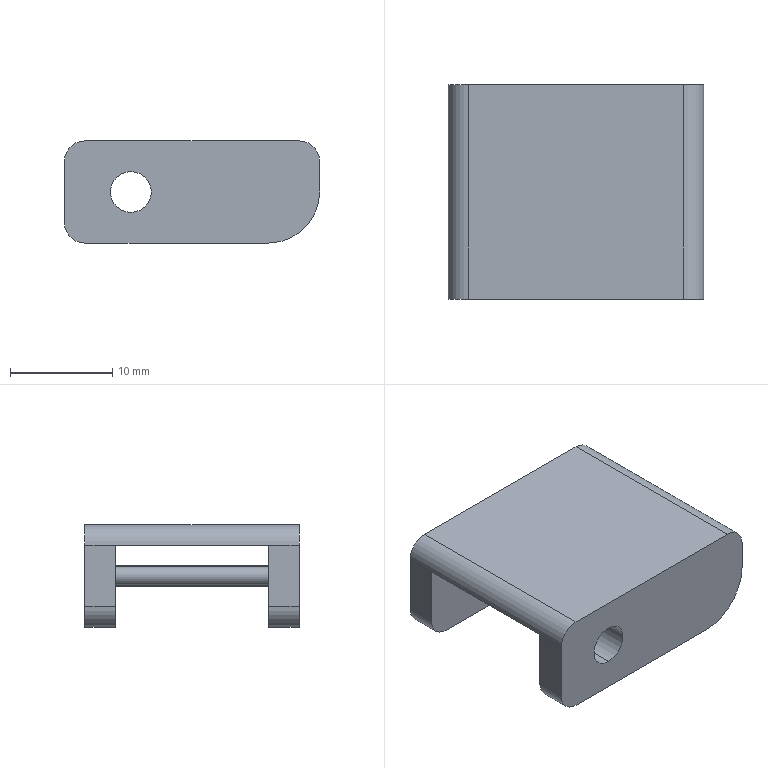Part | SolidWorks | features ICE 4, Fillet 2, Extrusion 1 | 1 solid | 26 faces | box 25 x 21 x 10 mm | volume 2190 mm3 | cylinder 14 | plane 12 | commonest cylinder face diameters 4 x8 1.809 x2 2.072 x2 10 x2
STEP:
#1=CARTESIAN_POINT('',(0.,7.5,-0.9044));
#2=VERTEX_POINT('',#1);
#3=CARTESIAN_POINT('',(0.,7.5,0.9044));
#4=VERTEX_POINT('',#3);
#5=CARTESIAN_POINT('',(0.,7.5,0.));
#6=DIRECTION('',(0.,-1.,0.));
#7=DIRECTION('',(0.,0.,1.));
#8=AXIS2_PLACEMENT_3D('',#5,#6,#7);
#9=CIRCLE('',#8,0.9044);
#10=EDGE_CURVE('',#2,#4,#9,.T.);
#11=ORIENTED_EDGE('',*,*,#10,.T.);
#12=CARTESIAN_POINT('',(0.,-7.5,0.9044));
#13=VERTEX_POINT('',#12);
#14=CARTESIAN_POINT('',(0.,10.058,0.9044));
#15=DIRECTION('',(0.,-1.,0.));
#16=VECTOR('',#15,1000.);
#17=LINE('',#14,#16);
#18=EDGE_CURVE('',#4,#13,#17,.T.);
#19=ORIENTED_EDGE('',*,*,#18,.T.);
#20=CARTESIAN_POINT('',(0.,-7.5,-0.9044));
#21=VERTEX_POINT('',#20);
#22=CARTESIAN_POINT('',(0.,-7.5,0.));
#23=DIRECTION('',(0.,1.,0.));
#24=DIRECTION('',(0.,0.,-1.));
#25=AXIS2_PLACEMENT_3D('',#22,#23,#24);
#26=CIRCLE('',#25,0.9044);
#27=EDGE_CURVE('',#13,#21,#26,.T.);
#28=ORIENTED_EDGE('',*,*,#27,.T.);
#29=CARTESIAN_POINT('',(0.,10.058,-0.9044));
#30=DIRECTION('',(0.,-1.,0.));
#31=VECTOR('',#30,1000.);
#32=LINE('',#29,#31);
#33=EDGE_CURVE('',#2,#21,#32,.T.);
#34=ORIENTED_EDGE('',*,*,#33,.F.);
#35=EDGE_LOOP('',(#11,#19,#28,#34));
#36=FACE_OUTER_BOUND('',#35,.T.);
#37=CARTESIAN_POINT('',(0.,10.058,0.));
#38=DIRECTION('',(0.,-1.,0.));
#39=DIRECTION('',(0.,0.,-1.));
#40=AXIS2_PLACEMENT_3D('',#37,#38,#39);
#41=CYLINDRICAL_SURFACE('',#40,0.9044);
#42=ADVANCED_FACE('',(#36),#41,.T.);
#43=CARTESIAN_POINT('',(4.,-7.5,1.036));
#44=VERTEX_POINT('',#43);
#45=CARTESIAN_POINT('',(4.,-7.5,-1.036));
#46=VERTEX_POINT('',#45);
#47=CARTESIAN_POINT('',(4.,-7.5,0.));
#48=DIRECTION('',(0.,1.,0.));
#49=DIRECTION('',(0.,0.,-1.));
#50=AXIS2_PLACEMENT_3D('',#47,#48,#49);
#51=CIRCLE('',#50,1.036);
#52=EDGE_CURVE('',#44,#46,#51,.T.);
#53=ORIENTED_EDGE('',*,*,#52,.T.);
#54=CARTESIAN_POINT('',(4.,7.5,-1.036));
#55=VERTEX_POINT('',#54);
#56=CARTESIAN_POINT('',(4.,-10.43,-1.036));
#57=DIRECTION('',(0.,1.,0.));
#58=VECTOR('',#57,1000.);
#59=LINE('',#56,#58);
#60=EDGE_CURVE('',#46,#55,#59,.T.);
#61=ORIENTED_EDGE('',*,*,#60,.T.);
#62=CARTESIAN_POINT('',(4.,7.5,1.036));
#63=VERTEX_POINT('',#62);
#64=CARTESIAN_POINT('',(4.,7.5,0.));
#65=DIRECTION('',(0.,1.,0.));
#66=DIRECTION('',(0.,0.,1.));
#67=AXIS2_PLACEMENT_3D('',#64,#65,#66);
#68=CIRCLE('',#67,1.036);
#69=EDGE_CURVE('',#63,#55,#68,.T.);
#70=ORIENTED_EDGE('',*,*,#69,.F.);
#71=CARTESIAN_POINT('',(4.,-10.43,1.036));
#72=DIRECTION('',(0.,1.,0.));
#73=VECTOR('',#72,1000.);
#74=LINE('',#71,#73);
#75=EDGE_CURVE('',#44,#63,#74,.T.);
#76=ORIENTED_EDGE('',*,*,#75,.F.);
#77=EDGE_LOOP('',(#53,#61,#70,#76));
#78=FACE_OUTER_BOUND('',#77,.T.);
#79=CARTESIAN_POINT('',(4.,-10.43,0.));
#80=DIRECTION('',(0.,1.,0.));
#81=DIRECTION('',(0.,0.,1.));
#82=AXIS2_PLACEMENT_3D('',#79,#80,#81);
#83=CYLINDRICAL_SURFACE('',#82,1.036);
#84=ADVANCED_FACE('',(#78),#83,.T.);
#85=CARTESIAN_POINT('',(-6.,-10.5,-2.));
#86=VERTEX_POINT('',#85);
#87=CARTESIAN_POINT('',(-6.,-10.5,2.));
#88=VERTEX_POINT('',#87);
#89=CARTESIAN_POINT('',(-6.,-10.5,0.));
#90=DIRECTION('',(0.,1.,0.));
#91=DIRECTION('',(0.,0.,1.));
#92=AXIS2_PLACEMENT_3D('',#89,#90,#91);
#93=CIRCLE('',#92,2.);
#94=EDGE_CURVE('',#86,#88,#93,.T.);
#95=ORIENTED_EDGE('',*,*,#94,.F.);
#96=CARTESIAN_POINT('',(-6.,-7.5,-2.));
#97=VERTEX_POINT('',#96);
#98=CARTESIAN_POINT('',(-6.,-10.5,-2.));
#99=DIRECTION('',(0.,1.,0.));
#100=VECTOR('',#99,1000.);
#101=LINE('',#98,#100);
#102=EDGE_CURVE('',#86,#97,#101,.T.);
#103=ORIENTED_EDGE('',*,*,#102,.T.);
#104=CARTESIAN_POINT('',(-6.,-7.5,2.));
#105=VERTEX_POINT('',#104);
#106=CARTESIAN_POINT('',(-6.,-7.5,0.));
#107=DIRECTION('',(0.,-1.,0.));
#108=DIRECTION('',(0.,0.,-1.));
#109=AXIS2_PLACEMENT_3D('',#106,#107,#108);
#110=CIRCLE('',#109,2.);
#111=EDGE_CURVE('',#105,#97,#110,.T.);
#112=ORIENTED_EDGE('',*,*,#111,.F.);
#113=CARTESIAN_POINT('',(-6.,-10.5,2.));
#114=DIRECTION('',(0.,1.,0.));
#115=VECTOR('',#114,1000.);
#116=LINE('',#113,#115);
#117=EDGE_CURVE('',#88,#105,#116,.T.);
#118=ORIENTED_EDGE('',*,*,#117,.F.);
#119=EDGE_LOOP('',(#95,#103,#112,#118));
#120=FACE_OUTER_BOUND('',#119,.T.);
#121=CARTESIAN_POINT('',(-6.,-10.5,0.));
#122=DIRECTION('',(0.,1.,0.));
#123=DIRECTION('',(0.,0.,1.));
#124=AXIS2_PLACEMENT_3D('',#121,#122,#123);
#125=CYLINDRICAL_SURFACE('',#124,2.);
#126=ADVANCED_FACE('',(#120),#125,.F.);
#127=CARTESIAN_POINT('',(-6.,7.5,-2.));
#128=VERTEX_POINT('',#127);
#129=CARTESIAN_POINT('',(-6.,7.5,2.));
#130=VERTEX_POINT('',#129);
#131=CARTESIAN_POINT('',(-6.,7.5,0.));
#132=DIRECTION('',(0.,1.,0.));
#133=DIRECTION('',(0.,0.,1.));
#134=AXIS2_PLACEMENT_3D('',#131,#132,#133);
#135=CIRCLE('',#134,2.);
#136=EDGE_CURVE('',#128,#130,#135,.T.);
#137=ORIENTED_EDGE('',*,*,#136,.F.);
#138=CARTESIAN_POINT('',(-6.,10.5,-2.));
#139=VERTEX_POINT('',#138);
#140=CARTESIAN_POINT('',(-6.,-10.5,-2.));
#141=DIRECTION('',(0.,1.,0.));
#142=VECTOR('',#141,1000.);
#143=LINE('',#140,#142);
#144=EDGE_CURVE('',#128,#139,#143,.T.);
#145=ORIENTED_EDGE('',*,*,#144,.T.);
#146=CARTESIAN_POINT('',(-6.,10.5,2.));
#147=VERTEX_POINT('',#146);
#148=CARTESIAN_POINT('',(-6.,10.5,0.));
#149=DIRECTION('',(0.,1.,0.));
#150=DIRECTION('',(0.,0.,1.));
#151=AXIS2_PLACEMENT_3D('',#148,#149,#150);
#152=CIRCLE('',#151,2.);
#153=EDGE_CURVE('',#139,#147,#152,.T.);
#154=ORIENTED_EDGE('',*,*,#153,.T.);
#155=CARTESIAN_POINT('',(-6.,-10.5,2.));
#156=DIRECTION('',(0.,1.,0.));
#157=VECTOR('',#156,1000.);
#158=LINE('',#155,#157);
#159=EDGE_CURVE('',#130,#147,#158,.T.);
#160=ORIENTED_EDGE('',*,*,#159,.F.);
#161=EDGE_LOOP('',(#137,#145,#154,#160));
#162=FACE_OUTER_BOUND('',#161,.T.);
#163=CARTESIAN_POINT('',(-6.,-10.5,0.));
#164=DIRECTION('',(0.,1.,0.));
#165=DIRECTION('',(0.,0.,1.));
#166=AXIS2_PLACEMENT_3D('',#163,#164,#165);
#167=CYLINDRICAL_SURFACE('',#166,2.);
#168=ADVANCED_FACE('',(#162),#167,.F.);
#169=CARTESIAN_POINT('',(12.5,7.5,0.));
#170=VERTEX_POINT('',#169);
#171=CARTESIAN_POINT('',(12.5,7.5,3.));
#172=VERTEX_POINT('',#171);
#173=CARTESIAN_POINT('',(12.5,7.5,-5.));
#174=DIRECTION('',(0.,0.,1.));
#175=VECTOR('',#174,1000.);
#176=LINE('',#173,#175);
#177=EDGE_CURVE('',#170,#172,#176,.T.);
#178=ORIENTED_EDGE('',*,*,#177,.F.);
#179=CARTESIAN_POINT('',(12.5,10.5,0.));
#180=VERTEX_POINT('',#179);
#181=CARTESIAN_POINT('',(12.5,10.5,0.));
#182=DIRECTION('',(0.,1.,0.));
#183=VECTOR('',#182,1000.);
#184=LINE('',#181,#183);
#185=EDGE_CURVE('',#170,#180,#184,.T.);
#186=ORIENTED_EDGE('',*,*,#185,.T.);
#187=CARTESIAN_POINT('',(12.5,10.5,3.));
#188=VERTEX_POINT('',#187);
#189=CARTESIAN_POINT('',(12.5,10.5,5.));
#190=DIRECTION('',(0.,0.,-1.));
#191=VECTOR('',#190,1000.);
#192=LINE('',#189,#191);
#193=EDGE_CURVE('',#188,#180,#192,.T.);
#194=ORIENTED_EDGE('',*,*,#193,.F.);
#195=CARTESIAN_POINT('',(12.5,10.5,3.));
#196=DIRECTION('',(0.,-1.,0.));
#197=VECTOR('',#196,1000.);
#198=LINE('',#195,#197);
#199=EDGE_CURVE('',#188,#172,#198,.T.);
#200=ORIENTED_EDGE('',*,*,#199,.T.);
#201=EDGE_LOOP('',(#178,#186,#194,#200));
#202=FACE_OUTER_BOUND('',#201,.T.);
#203=CARTESIAN_POINT('',(12.5,10.5,5.));
#204=DIRECTION('',(-1.,0.,0.));
#205=DIRECTION('',(0.,0.,1.));
#206=AXIS2_PLACEMENT_3D('',#203,#204,#205);
#207=PLANE('',#206);
#208=ADVANCED_FACE('',(#202),#207,.F.);
#209=CARTESIAN_POINT('',(-12.5,-10.5,-3.));
#210=VERTEX_POINT('',#209);
#211=CARTESIAN_POINT('',(-12.5,-10.5,3.));
#212=VERTEX_POINT('',#211);
#213=CARTESIAN_POINT('',(-12.5,-10.5,5.));
#214=DIRECTION('',(0.,0.,1.));
#215=VECTOR('',#214,1000.);
#216=LINE('',#213,#215);
#217=EDGE_CURVE('',#210,#212,#216,.T.);
#218=ORIENTED_EDGE('',*,*,#217,.T.);
#219=CARTESIAN_POINT('',(-12.5,-7.5,3.));
#220=VERTEX_POINT('',#219);
#221=CARTESIAN_POINT('',(-12.5,10.5,3.));
#222=DIRECTION('',(0.,1.,0.));
#223=VECTOR('',#222,1000.);
#224=LINE('',#221,#223);
#225=EDGE_CURVE('',#212,#220,#224,.T.);
#226=ORIENTED_EDGE('',*,*,#225,.T.);
#227=CARTESIAN_POINT('',(-12.5,-7.5,-3.));
#228=VERTEX_POINT('',#227);
#229=CARTESIAN_POINT('',(-12.5,-7.5,-5.));
#230=DIRECTION('',(0.,0.,-1.));
#231=VECTOR('',#230,1000.);
#232=LINE('',#229,#231);
#233=EDGE_CURVE('',#220,#228,#232,.T.);
#234=ORIENTED_EDGE('',*,*,#233,.T.);
#235=CARTESIAN_POINT('',(-12.5,10.5,-3.));
#236=DIRECTION('',(0.,-1.,0.));
#237=VECTOR('',#236,1000.);
#238=LINE('',#235,#237);
#239=EDGE_CURVE('',#228,#210,#238,.T.);
#240=ORIENTED_EDGE('',*,*,#239,.T.);
#241=EDGE_LOOP('',(#218,#226,#234,#240));
#242=FACE_OUTER_BOUND('',#241,.T.);
#243=CARTESIAN_POINT('',(-12.5,10.5,5.));
#244=DIRECTION('',(1.,0.,0.));
#245=DIRECTION('',(0.,0.,-1.));
#246=AXIS2_PLACEMENT_3D('',#243,#244,#245);
#247=PLANE('',#246);
#248=ADVANCED_FACE('',(#242),#247,.F.);
#249=CARTESIAN_POINT('',(-10.5,-7.5,-5.));
#250=VERTEX_POINT('',#249);
#251=CARTESIAN_POINT('',(7.5,-7.5,-5.));
#252=VERTEX_POINT('',#251);
#253=CARTESIAN_POINT('',(-12.5,-7.5,-5.));
#254=DIRECTION('',(1.,0.,0.));
#255=VECTOR('',#254,1000.);
#256=LINE('',#253,#255);
#257=EDGE_CURVE('',#250,#252,#256,.T.);
#258=ORIENTED_EDGE('',*,*,#257,.T.);
#259=CARTESIAN_POINT('',(7.5,-10.5,-5.));
#260=VERTEX_POINT('',#259);
#261=CARTESIAN_POINT('',(7.5,10.5,-5.));
#262=DIRECTION('',(0.,-1.,0.));
#263=VECTOR('',#262,1000.);
#264=LINE('',#261,#263);
#265=EDGE_CURVE('',#252,#260,#264,.T.);
#266=ORIENTED_EDGE('',*,*,#265,.T.);
#267=CARTESIAN_POINT('',(-10.5,-10.5,-5.));
#268=VERTEX_POINT('',#267);
#269=CARTESIAN_POINT('',(-12.5,-10.5,-5.));
#270=DIRECTION('',(-1.,0.,0.));
#271=VECTOR('',#270,1000.);
#272=LINE('',#269,#271);
#273=EDGE_CURVE('',#260,#268,#272,.T.);
#274=ORIENTED_EDGE('',*,*,#273,.T.);
#275=CARTESIAN_POINT('',(-10.5,10.5,-5.));
#276=DIRECTION('',(0.,1.,0.));
#277=VECTOR('',#276,1000.);
#278=LINE('',#275,#277);
#279=EDGE_CURVE('',#268,#250,#278,.T.);
#280=ORIENTED_EDGE('',*,*,#279,.T.);
#281=EDGE_LOOP('',(#258,#266,#274,#280));
#282=FACE_OUTER_BOUND('',#281,.T.);
#283=CARTESIAN_POINT('',(-12.5,10.5,-5.));
#284=DIRECTION('',(0.,0.,1.));
#285=DIRECTION('',(1.,0.,0.));
#286=AXIS2_PLACEMENT_3D('',#283,#284,#285);
#287=PLANE('',#286);
#288=ADVANCED_FACE('',(#282),#287,.F.);
#289=CARTESIAN_POINT('',(12.5,-10.5,3.));
#290=VERTEX_POINT('',#289);
#291=CARTESIAN_POINT('',(12.5,-10.5,0.));
#292=VERTEX_POINT('',#291);
#293=CARTESIAN_POINT('',(12.5,-10.5,5.));
#294=DIRECTION('',(0.,0.,-1.));
#295=VECTOR('',#294,1000.);
#296=LINE('',#293,#295);
#297=EDGE_CURVE('',#290,#292,#296,.T.);
#298=ORIENTED_EDGE('',*,*,#297,.T.);
#299=CARTESIAN_POINT('',(12.5,-7.5,0.));
#300=VERTEX_POINT('',#299);
#301=CARTESIAN_POINT('',(12.5,10.5,0.));
#302=DIRECTION('',(0.,1.,0.));
#303=VECTOR('',#302,1000.);
#304=LINE('',#301,#303);
#305=EDGE_CURVE('',#292,#300,#304,.T.);
#306=ORIENTED_EDGE('',*,*,#305,.T.);
#307=CARTESIAN_POINT('',(12.5,-7.5,3.));
#308=VERTEX_POINT('',#307);
#309=CARTESIAN_POINT('',(12.5,-7.5,-5.));
#310=DIRECTION('',(0.,0.,-1.));
#311=VECTOR('',#310,1000.);
#312=LINE('',#309,#311);
#313=EDGE_CURVE('',#308,#300,#312,.T.);
#314=ORIENTED_EDGE('',*,*,#313,.F.);
#315=CARTESIAN_POINT('',(12.5,10.5,3.));
#316=DIRECTION('',(0.,-1.,0.));
#317=VECTOR('',#316,1000.);
#318=LINE('',#315,#317);
#319=EDGE_CURVE('',#308,#290,#318,.T.);
#320=ORIENTED_EDGE('',*,*,#319,.T.);
#321=EDGE_LOOP('',(#298,#306,#314,#320));
#322=FACE_OUTER_BOUND('',#321,.T.);
#323=CARTESIAN_POINT('',(12.5,10.5,5.));
#324=DIRECTION('',(-1.,0.,0.));
#325=DIRECTION('',(0.,0.,1.));
#326=AXIS2_PLACEMENT_3D('',#323,#324,#325);
#327=PLANE('',#326);
#328=ADVANCED_FACE('',(#322),#327,.F.);
#329=CARTESIAN_POINT('',(7.5,10.5,-5.));
#330=VERTEX_POINT('',#329);
#331=CARTESIAN_POINT('',(-10.5,10.5,-5.));
#332=VERTEX_POINT('',#331);
#333=CARTESIAN_POINT('',(-12.5,10.5,-5.));
#334=DIRECTION('',(-1.,0.,0.));
#335=VECTOR('',#334,1000.);
#336=LINE('',#333,#335);
#337=EDGE_CURVE('',#330,#332,#336,.T.);
#338=ORIENTED_EDGE('',*,*,#337,.F.);
#339=CARTESIAN_POINT('',(7.5,7.5,-5.));
#340=VERTEX_POINT('',#339);
#341=CARTESIAN_POINT('',(7.5,10.5,-5.));
#342=DIRECTION('',(0.,-1.,0.));
#343=VECTOR('',#342,1000.);
#344=LINE('',#341,#343);
#345=EDGE_CURVE('',#330,#340,#344,.T.);
#346=ORIENTED_EDGE('',*,*,#345,.T.);
#347=CARTESIAN_POINT('',(-10.5,7.5,-5.));
#348=VERTEX_POINT('',#347);
#349=CARTESIAN_POINT('',(-12.5,7.5,-5.));
#350=DIRECTION('',(1.,0.,0.));
#351=VECTOR('',#350,1000.);
#352=LINE('',#349,#351);
#353=EDGE_CURVE('',#348,#340,#352,.T.);
#354=ORIENTED_EDGE('',*,*,#353,.F.);
#355=CARTESIAN_POINT('',(-10.5,10.5,-5.));
#356=DIRECTION('',(0.,1.,0.));
#357=VECTOR('',#356,1000.);
#358=LINE('',#355,#357);
#359=EDGE_CURVE('',#348,#332,#358,.T.);
#360=ORIENTED_EDGE('',*,*,#359,.T.);
#361=EDGE_LOOP('',(#338,#346,#354,#360));
#362=FACE_OUTER_BOUND('',#361,.T.);
#363=CARTESIAN_POINT('',(-12.5,10.5,-5.));
#364=DIRECTION('',(0.,0.,1.));
#365=DIRECTION('',(1.,0.,0.));
#366=AXIS2_PLACEMENT_3D('',#363,#364,#365);
#367=PLANE('',#366);
#368=ADVANCED_FACE('',(#362),#367,.F.);
#369=CARTESIAN_POINT('',(-12.5,7.5,-3.));
#370=VERTEX_POINT('',#369);
#371=CARTESIAN_POINT('',(-12.5,7.5,3.));
#372=VERTEX_POINT('',#371);
#373=CARTESIAN_POINT('',(-12.5,7.5,-5.));
#374=DIRECTION('',(0.,0.,1.));
#375=VECTOR('',#374,1000.);
#376=LINE('',#373,#375);
#377=EDGE_CURVE('',#370,#372,#376,.T.);
#378=ORIENTED_EDGE('',*,*,#377,.T.);
#379=CARTESIAN_POINT('',(-12.5,10.5,3.));
#380=VERTEX_POINT('',#379);
#381=CARTESIAN_POINT('',(-12.5,10.5,3.));
#382=DIRECTION('',(0.,1.,0.));
#383=VECTOR('',#382,1000.);
#384=LINE('',#381,#383);
#385=EDGE_CURVE('',#372,#380,#384,.T.);
#386=ORIENTED_EDGE('',*,*,#385,.T.);
#387=CARTESIAN_POINT('',(-12.5,10.5,-3.));
#388=VERTEX_POINT('',#387);
#389=CARTESIAN_POINT('',(-12.5,10.5,5.));
#390=DIRECTION('',(0.,0.,1.));
#391=VECTOR('',#390,1000.);
#392=LINE('',#389,#391);
#393=EDGE_CURVE('',#388,#380,#392,.T.);
#394=ORIENTED_EDGE('',*,*,#393,.F.);
#395=CARTESIAN_POINT('',(-12.5,10.5,-3.));
#396=DIRECTION('',(0.,-1.,0.));
#397=VECTOR('',#396,1000.);
#398=LINE('',#395,#397);
#399=EDGE_CURVE('',#388,#370,#398,.T.);
#400=ORIENTED_EDGE('',*,*,#399,.T.);
#401=EDGE_LOOP('',(#378,#386,#394,#400));
#402=FACE_OUTER_BOUND('',#401,.T.);
#403=CARTESIAN_POINT('',(-12.5,10.5,5.));
#404=DIRECTION('',(1.,0.,0.));
#405=DIRECTION('',(0.,0.,-1.));
#406=AXIS2_PLACEMENT_3D('',#403,#404,#405);
#407=PLANE('',#406);
#408=ADVANCED_FACE('',(#402),#407,.F.);
#409=CARTESIAN_POINT('',(-10.5,10.5,5.));
#410=VERTEX_POINT('',#409);
#411=CARTESIAN_POINT('',(10.5,10.5,5.));
#412=VERTEX_POINT('',#411);
#413=CARTESIAN_POINT('',(-12.5,10.5,5.));
#414=DIRECTION('',(1.,0.,0.));
#415=VECTOR('',#414,1000.);
#416=LINE('',#413,#415);
#417=EDGE_CURVE('',#410,#412,#416,.T.);
#418=ORIENTED_EDGE('',*,*,#417,.F.);
#419=CARTESIAN_POINT('',(-10.5,-10.5,5.));
#420=VERTEX_POINT('',#419);
#421=CARTESIAN_POINT('',(-10.5,10.5,5.));
#422=DIRECTION('',(0.,-1.,0.));
#423=VECTOR('',#422,1000.);
#424=LINE('',#421,#423);
#425=EDGE_CURVE('',#410,#420,#424,.T.);
#426=ORIENTED_EDGE('',*,*,#425,.T.);
#427=CARTESIAN_POINT('',(10.5,-10.5,5.));
#428=VERTEX_POINT('',#427);
#429=CARTESIAN_POINT('',(-12.5,-10.5,5.));
#430=DIRECTION('',(1.,0.,0.));
#431=VECTOR('',#430,1000.);
#432=LINE('',#429,#431);
#433=EDGE_CURVE('',#420,#428,#432,.T.);
#434=ORIENTED_EDGE('',*,*,#433,.T.);
#435=CARTESIAN_POINT('',(10.5,10.5,5.));
#436=DIRECTION('',(0.,1.,0.));
#437=VECTOR('',#436,1000.);
#438=LINE('',#435,#437);
#439=EDGE_CURVE('',#428,#412,#438,.T.);
#440=ORIENTED_EDGE('',*,*,#439,.T.);
#441=EDGE_LOOP('',(#418,#426,#434,#440));
#442=FACE_OUTER_BOUND('',#441,.T.);
#443=CARTESIAN_POINT('',(-12.5,10.5,5.));
#444=DIRECTION('',(0.,0.,-1.));
#445=DIRECTION('',(-1.,0.,0.));
#446=AXIS2_PLACEMENT_3D('',#443,#444,#445);
#447=PLANE('',#446);
#448=ADVANCED_FACE('',(#442),#447,.F.);
#449=CARTESIAN_POINT('',(-6.,10.5,0.));
#450=DIRECTION('',(0.,1.,0.));
#451=DIRECTION('',(0.,0.,1.));
#452=AXIS2_PLACEMENT_3D('',#449,#450,#451);
#453=CIRCLE('',#452,2.);
#454=EDGE_CURVE('',#147,#139,#453,.T.);
#455=ORIENTED_EDGE('',*,*,#454,.F.);
#456=ORIENTED_EDGE('',*,*,#153,.F.);
#457=EDGE_LOOP('',(#455,#456));
#458=FACE_BOUND('',#457,.T.);
#459=ORIENTED_EDGE('',*,*,#193,.T.);
#460=CARTESIAN_POINT('',(7.5,10.5,0.));
#461=DIRECTION('',(0.,1.,0.));
#462=DIRECTION('',(0.,0.,-1.));
#463=AXIS2_PLACEMENT_3D('',#460,#461,#462);
#464=CIRCLE('',#463,5.);
#465=EDGE_CURVE('',#180,#330,#464,.T.);
#466=ORIENTED_EDGE('',*,*,#465,.T.);
#467=ORIENTED_EDGE('',*,*,#337,.T.);
#468=CARTESIAN_POINT('',(-10.5,10.5,-3.));
#469=DIRECTION('',(0.,1.,0.));
#470=DIRECTION('',(0.,0.,-1.));
#471=AXIS2_PLACEMENT_3D('',#468,#469,#470);
#472=CIRCLE('',#471,2.);
#473=EDGE_CURVE('',#332,#388,#472,.T.);
#474=ORIENTED_EDGE('',*,*,#473,.T.);
#475=ORIENTED_EDGE('',*,*,#393,.T.);
#476=CARTESIAN_POINT('',(-10.5,10.5,3.));
#477=DIRECTION('',(0.,1.,0.));
#478=DIRECTION('',(0.,0.,-1.));
#479=AXIS2_PLACEMENT_3D('',#476,#477,#478);
#480=CIRCLE('',#479,2.);
#481=EDGE_CURVE('',#380,#410,#480,.T.);
#482=ORIENTED_EDGE('',*,*,#481,.T.);
#483=ORIENTED_EDGE('',*,*,#417,.T.);
#484=CARTESIAN_POINT('',(10.5,10.5,3.));
#485=DIRECTION('',(0.,1.,0.));
#486=DIRECTION('',(0.,0.,-1.));
#487=AXIS2_PLACEMENT_3D('',#484,#485,#486);
#488=CIRCLE('',#487,2.);
#489=EDGE_CURVE('',#412,#188,#488,.T.);
#490=ORIENTED_EDGE('',*,*,#489,.T.);
#491=EDGE_LOOP('',(#459,#466,#467,#474,#475,#482,#483,#490));
#492=FACE_OUTER_BOUND('',#491,.T.);
#493=CARTESIAN_POINT('',(0.,10.5,0.));
#494=DIRECTION('',(0.,-1.,0.));
#495=DIRECTION('',(0.,0.,-1.));
#496=AXIS2_PLACEMENT_3D('',#493,#494,#495);
#497=PLANE('',#496);
#498=ADVANCED_FACE('',(#458,#492),#497,.F.);
#499=CARTESIAN_POINT('',(-6.,-10.5,0.));
#500=DIRECTION('',(0.,1.,0.));
#501=DIRECTION('',(0.,0.,1.));
#502=AXIS2_PLACEMENT_3D('',#499,#500,#501);
#503=CIRCLE('',#502,2.);
#504=EDGE_CURVE('',#88,#86,#503,.T.);
#505=ORIENTED_EDGE('',*,*,#504,.T.);
#506=ORIENTED_EDGE('',*,*,#94,.T.);
#507=EDGE_LOOP('',(#505,#506));
#508=FACE_BOUND('',#507,.T.);
#509=ORIENTED_EDGE('',*,*,#273,.F.);
#510=CARTESIAN_POINT('',(7.5,-10.5,0.));
#511=DIRECTION('',(0.,-1.,0.));
#512=DIRECTION('',(0.,0.,-1.));
#513=AXIS2_PLACEMENT_3D('',#510,#511,#512);
#514=CIRCLE('',#513,5.);
#515=EDGE_CURVE('',#260,#292,#514,.T.);
#516=ORIENTED_EDGE('',*,*,#515,.T.);
#517=ORIENTED_EDGE('',*,*,#297,.F.);
#518=CARTESIAN_POINT('',(10.5,-10.5,3.));
#519=DIRECTION('',(0.,-1.,0.));
#520=DIRECTION('',(0.,0.,-1.));
#521=AXIS2_PLACEMENT_3D('',#518,#519,#520);
#522=CIRCLE('',#521,2.);
#523=EDGE_CURVE('',#290,#428,#522,.T.);
#524=ORIENTED_EDGE('',*,*,#523,.T.);
#525=ORIENTED_EDGE('',*,*,#433,.F.);
#526=CARTESIAN_POINT('',(-10.5,-10.5,3.));
#527=DIRECTION('',(0.,-1.,0.));
#528=DIRECTION('',(0.,0.,-1.));
#529=AXIS2_PLACEMENT_3D('',#526,#527,#528);
#530=CIRCLE('',#529,2.);
#531=EDGE_CURVE('',#420,#212,#530,.T.);
#532=ORIENTED_EDGE('',*,*,#531,.T.);
#533=ORIENTED_EDGE('',*,*,#217,.F.);
#534=CARTESIAN_POINT('',(-10.5,-10.5,-3.));
#535=DIRECTION('',(0.,-1.,0.));
#536=DIRECTION('',(0.,0.,-1.));
#537=AXIS2_PLACEMENT_3D('',#534,#535,#536);
#538=CIRCLE('',#537,2.);
#539=EDGE_CURVE('',#210,#268,#538,.T.);
#540=ORIENTED_EDGE('',*,*,#539,.T.);
#541=EDGE_LOOP('',(#509,#516,#517,#524,#525,#532,#533,#540));
#542=FACE_OUTER_BOUND('',#541,.T.);
#543=CARTESIAN_POINT('',(0.,-10.5,0.));
#544=DIRECTION('',(0.,-1.,0.));
#545=DIRECTION('',(0.,0.,-1.));
#546=AXIS2_PLACEMENT_3D('',#543,#544,#545);
#547=PLANE('',#546);
#548=ADVANCED_FACE('',(#508,#542),#547,.T.);
#549=CARTESIAN_POINT('',(0.,-7.5,0.));
#550=DIRECTION('',(0.,1.,0.));
#551=DIRECTION('',(0.,0.,-1.));
#552=AXIS2_PLACEMENT_3D('',#549,#550,#551);
#553=CIRCLE('',#552,0.9044);
#554=EDGE_CURVE('',#21,#13,#553,.T.);
#555=ORIENTED_EDGE('',*,*,#554,.F.);
#556=ORIENTED_EDGE('',*,*,#27,.F.);
#557=EDGE_LOOP('',(#555,#556));
#558=FACE_BOUND('',#557,.T.);
#559=ORIENTED_EDGE('',*,*,#52,.F.);
#560=CARTESIAN_POINT('',(4.,-7.5,0.));
#561=DIRECTION('',(0.,1.,0.));
#562=DIRECTION('',(0.,0.,-1.));
#563=AXIS2_PLACEMENT_3D('',#560,#561,#562);
#564=CIRCLE('',#563,1.036);
#565=EDGE_CURVE('',#46,#44,#564,.T.);
#566=ORIENTED_EDGE('',*,*,#565,.F.);
#567=EDGE_LOOP('',(#559,#566));
#568=FACE_BOUND('',#567,.T.);
#569=ORIENTED_EDGE('',*,*,#111,.T.);
#570=CARTESIAN_POINT('',(-6.,-7.5,0.));
#571=DIRECTION('',(0.,-1.,0.));
#572=DIRECTION('',(0.,0.,-1.));
#573=AXIS2_PLACEMENT_3D('',#570,#571,#572);
#574=CIRCLE('',#573,2.);
#575=EDGE_CURVE('',#97,#105,#574,.T.);
#576=ORIENTED_EDGE('',*,*,#575,.T.);
#577=EDGE_LOOP('',(#569,#576));
#578=FACE_BOUND('',#577,.T.);
#579=ORIENTED_EDGE('',*,*,#313,.T.);
#580=CARTESIAN_POINT('',(7.5,-7.5,0.));
#581=DIRECTION('',(0.,1.,0.));
#582=DIRECTION('',(0.,0.,-1.));
#583=AXIS2_PLACEMENT_3D('',#580,#581,#582);
#584=CIRCLE('',#583,5.);
#585=EDGE_CURVE('',#300,#252,#584,.T.);
#586=ORIENTED_EDGE('',*,*,#585,.T.);
#587=ORIENTED_EDGE('',*,*,#257,.F.);
#588=CARTESIAN_POINT('',(-10.5,-7.5,-3.));
#589=DIRECTION('',(0.,1.,0.));
#590=DIRECTION('',(0.,0.,-1.));
#591=AXIS2_PLACEMENT_3D('',#588,#589,#590);
#592=CIRCLE('',#591,2.);
#593=EDGE_CURVE('',#250,#228,#592,.T.);
#594=ORIENTED_EDGE('',*,*,#593,.T.);
#595=ORIENTED_EDGE('',*,*,#233,.F.);
#596=CARTESIAN_POINT('',(-12.5,-7.5,3.));
#597=DIRECTION('',(1.,0.,0.));
#598=VECTOR('',#597,1000.);
#599=LINE('',#596,#598);
#600=EDGE_CURVE('',#220,#308,#599,.T.);
#601=ORIENTED_EDGE('',*,*,#600,.T.);
#602=EDGE_LOOP('',(#579,#586,#587,#594,#595,#601));
#603=FACE_OUTER_BOUND('',#602,.T.);
#604=CARTESIAN_POINT('',(-12.5,-7.5,-5.));
#605=DIRECTION('',(0.,-1.,0.));
#606=DIRECTION('',(0.,0.,-1.));
#607=AXIS2_PLACEMENT_3D('',#604,#605,#606);
#608=PLANE('',#607);
#609=ADVANCED_FACE('',(#558,#568,#578,#603),#608,.F.);
#610=CARTESIAN_POINT('',(12.5,-7.5,3.));
#611=DIRECTION('',(0.,-1.,0.));
#612=VECTOR('',#611,1000.);
#613=LINE('',#610,#612);
#614=EDGE_CURVE('',#172,#308,#613,.T.);
#615=ORIENTED_EDGE('',*,*,#614,.T.);
#616=ORIENTED_EDGE('',*,*,#600,.F.);
#617=CARTESIAN_POINT('',(-12.5,-7.5,3.));
#618=DIRECTION('',(0.,-1.,0.));
#619=VECTOR('',#618,1000.);
#620=LINE('',#617,#619);
#621=EDGE_CURVE('',#372,#220,#620,.T.);
#622=ORIENTED_EDGE('',*,*,#621,.F.);
#623=CARTESIAN_POINT('',(-12.5,7.5,3.));
#624=DIRECTION('',(1.,0.,0.));
#625=VECTOR('',#624,1000.);
#626=LINE('',#623,#625);
#627=EDGE_CURVE('',#372,#172,#626,.T.);
#628=ORIENTED_EDGE('',*,*,#627,.T.);
#629=EDGE_LOOP('',(#615,#616,#622,#628));
#630=FACE_OUTER_BOUND('',#629,.T.);
#631=CARTESIAN_POINT('',(-12.5,-7.5,3.));
#632=DIRECTION('',(0.,0.,1.));
#633=DIRECTION('',(1.,0.,0.));
#634=AXIS2_PLACEMENT_3D('',#631,#632,#633);
#635=PLANE('',#634);
#636=ADVANCED_FACE('',(#630),#635,.F.);
#637=ORIENTED_EDGE('',*,*,#10,.F.);
#638=CARTESIAN_POINT('',(0.,7.5,0.));
#639=DIRECTION('',(0.,-1.,0.));
#640=DIRECTION('',(0.,0.,1.));
#641=AXIS2_PLACEMENT_3D('',#638,#639,#640);
#642=CIRCLE('',#641,0.9044);
#643=EDGE_CURVE('',#4,#2,#642,.T.);
#644=ORIENTED_EDGE('',*,*,#643,.F.);
#645=EDGE_LOOP('',(#637,#644));
#646=FACE_BOUND('',#645,.T.);
#647=ORIENTED_EDGE('',*,*,#69,.T.);
#648=CARTESIAN_POINT('',(4.,7.5,0.));
#649=DIRECTION('',(0.,1.,0.));
#650=DIRECTION('',(0.,0.,1.));
#651=AXIS2_PLACEMENT_3D('',#648,#649,#650);
#652=CIRCLE('',#651,1.036);
#653=EDGE_CURVE('',#55,#63,#652,.T.);
#654=ORIENTED_EDGE('',*,*,#653,.T.);
#655=EDGE_LOOP('',(#647,#654));
#656=FACE_BOUND('',#655,.T.);
#657=CARTESIAN_POINT('',(-6.,7.5,0.));
#658=DIRECTION('',(0.,1.,0.));
#659=DIRECTION('',(0.,0.,1.));
#660=AXIS2_PLACEMENT_3D('',#657,#658,#659);
#661=CIRCLE('',#660,2.);
#662=EDGE_CURVE('',#130,#128,#661,.T.);
#663=ORIENTED_EDGE('',*,*,#662,.T.);
#664=ORIENTED_EDGE('',*,*,#136,.T.);
#665=EDGE_LOOP('',(#663,#664));
#666=FACE_BOUND('',#665,.T.);
#667=ORIENTED_EDGE('',*,*,#353,.T.);
#668=CARTESIAN_POINT('',(7.5,7.5,0.));
#669=DIRECTION('',(0.,-1.,0.));
#670=DIRECTION('',(0.,0.,1.));
#671=AXIS2_PLACEMENT_3D('',#668,#669,#670);
#672=CIRCLE('',#671,5.);
#673=EDGE_CURVE('',#340,#170,#672,.T.);
#674=ORIENTED_EDGE('',*,*,#673,.T.);
#675=ORIENTED_EDGE('',*,*,#177,.T.);
#676=ORIENTED_EDGE('',*,*,#627,.F.);
#677=ORIENTED_EDGE('',*,*,#377,.F.);
#678=CARTESIAN_POINT('',(-10.5,7.5,-3.));
#679=DIRECTION('',(0.,-1.,0.));
#680=DIRECTION('',(0.,0.,1.));
#681=AXIS2_PLACEMENT_3D('',#678,#679,#680);
#682=CIRCLE('',#681,2.);
#683=EDGE_CURVE('',#370,#348,#682,.T.);
#684=ORIENTED_EDGE('',*,*,#683,.T.);
#685=EDGE_LOOP('',(#667,#674,#675,#676,#677,#684));
#686=FACE_OUTER_BOUND('',#685,.T.);
#687=CARTESIAN_POINT('',(-12.5,7.5,-5.));
#688=DIRECTION('',(0.,1.,0.));
#689=DIRECTION('',(0.,0.,1.));
#690=AXIS2_PLACEMENT_3D('',#687,#688,#689);
#691=PLANE('',#690);
#692=ADVANCED_FACE('',(#646,#656,#666,#686),#691,.F.);
#693=ORIENTED_EDGE('',*,*,#621,.T.);
#694=ORIENTED_EDGE('',*,*,#225,.F.);
#695=ORIENTED_EDGE('',*,*,#531,.F.);
#696=ORIENTED_EDGE('',*,*,#425,.F.);
#697=ORIENTED_EDGE('',*,*,#481,.F.);
#698=ORIENTED_EDGE('',*,*,#385,.F.);
#699=EDGE_LOOP('',(#693,#694,#695,#696,#697,#698));
#700=FACE_OUTER_BOUND('',#699,.T.);
#701=CARTESIAN_POINT('',(-10.5,10.5,3.));
#702=DIRECTION('',(0.,-1.,0.));
#703=DIRECTION('',(0.,0.,-1.));
#704=AXIS2_PLACEMENT_3D('',#701,#702,#703);
#705=CYLINDRICAL_SURFACE('',#704,2.);
#706=ADVANCED_FACE('',(#700),#705,.T.);
#707=ORIENTED_EDGE('',*,*,#489,.F.);
#708=ORIENTED_EDGE('',*,*,#439,.F.);
#709=ORIENTED_EDGE('',*,*,#523,.F.);
#710=ORIENTED_EDGE('',*,*,#319,.F.);
#711=ORIENTED_EDGE('',*,*,#614,.F.);
#712=ORIENTED_EDGE('',*,*,#199,.F.);
#713=EDGE_LOOP('',(#707,#708,#709,#710,#711,#712));
#714=FACE_OUTER_BOUND('',#713,.T.);
#715=CARTESIAN_POINT('',(10.5,10.5,3.));
#716=DIRECTION('',(0.,-1.,0.));
#717=DIRECTION('',(0.,0.,-1.));
#718=AXIS2_PLACEMENT_3D('',#715,#716,#717);
#719=CYLINDRICAL_SURFACE('',#718,2.);
#720=ADVANCED_FACE('',(#714),#719,.T.);
#721=ORIENTED_EDGE('',*,*,#593,.F.);
#722=ORIENTED_EDGE('',*,*,#279,.F.);
#723=ORIENTED_EDGE('',*,*,#539,.F.);
#724=ORIENTED_EDGE('',*,*,#239,.F.);
#725=EDGE_LOOP('',(#721,#722,#723,#724));
#726=FACE_OUTER_BOUND('',#725,.T.);
#727=CARTESIAN_POINT('',(-10.5,10.5,-3.));
#728=DIRECTION('',(0.,-1.,0.));
#729=DIRECTION('',(0.,0.,-1.));
#730=AXIS2_PLACEMENT_3D('',#727,#728,#729);
#731=CYLINDRICAL_SURFACE('',#730,2.);
#732=ADVANCED_FACE('',(#726),#731,.T.);
#733=ORIENTED_EDGE('',*,*,#473,.F.);
#734=ORIENTED_EDGE('',*,*,#359,.F.);
#735=ORIENTED_EDGE('',*,*,#683,.F.);
#736=ORIENTED_EDGE('',*,*,#399,.F.);
#737=EDGE_LOOP('',(#733,#734,#735,#736));
#738=FACE_OUTER_BOUND('',#737,.T.);
#739=CARTESIAN_POINT('',(-10.5,10.5,-3.));
#740=DIRECTION('',(0.,-1.,0.));
#741=DIRECTION('',(0.,0.,-1.));
#742=AXIS2_PLACEMENT_3D('',#739,#740,#741);
#743=CYLINDRICAL_SURFACE('',#742,2.);
#744=ADVANCED_FACE('',(#738),#743,.T.);
#745=ORIENTED_EDGE('',*,*,#585,.F.);
#746=ORIENTED_EDGE('',*,*,#305,.F.);
#747=ORIENTED_EDGE('',*,*,#515,.F.);
#748=ORIENTED_EDGE('',*,*,#265,.F.);
#749=EDGE_LOOP('',(#745,#746,#747,#748));
#750=FACE_OUTER_BOUND('',#749,.T.);
#751=CARTESIAN_POINT('',(7.5,10.5,0.));
#752=DIRECTION('',(0.,-1.,0.));
#753=DIRECTION('',(0.,0.,-1.));
#754=AXIS2_PLACEMENT_3D('',#751,#752,#753);
#755=CYLINDRICAL_SURFACE('',#754,5.);
#756=ADVANCED_FACE('',(#750),#755,.T.);
#757=ORIENTED_EDGE('',*,*,#465,.F.);
#758=ORIENTED_EDGE('',*,*,#185,.F.);
#759=ORIENTED_EDGE('',*,*,#673,.F.);
#760=ORIENTED_EDGE('',*,*,#345,.F.);
#761=EDGE_LOOP('',(#757,#758,#759,#760));
#762=FACE_OUTER_BOUND('',#761,.T.);
#763=CARTESIAN_POINT('',(7.5,10.5,0.));
#764=DIRECTION('',(0.,-1.,0.));
#765=DIRECTION('',(0.,0.,-1.));
#766=AXIS2_PLACEMENT_3D('',#763,#764,#765);
#767=CYLINDRICAL_SURFACE('',#766,5.);
#768=ADVANCED_FACE('',(#762),#767,.T.);
#769=ORIENTED_EDGE('',*,*,#144,.F.);
#770=ORIENTED_EDGE('',*,*,#662,.F.);
#771=ORIENTED_EDGE('',*,*,#159,.T.);
#772=ORIENTED_EDGE('',*,*,#454,.T.);
#773=EDGE_LOOP('',(#769,#770,#771,#772));
#774=FACE_OUTER_BOUND('',#773,.T.);
#775=CARTESIAN_POINT('',(-6.,-10.5,0.));
#776=DIRECTION('',(0.,1.,0.));
#777=DIRECTION('',(0.,0.,1.));
#778=AXIS2_PLACEMENT_3D('',#775,#776,#777);
#779=CYLINDRICAL_SURFACE('',#778,2.);
#780=ADVANCED_FACE('',(#774),#779,.F.);
#781=ORIENTED_EDGE('',*,*,#102,.F.);
#782=ORIENTED_EDGE('',*,*,#504,.F.);
#783=ORIENTED_EDGE('',*,*,#117,.T.);
#784=ORIENTED_EDGE('',*,*,#575,.F.);
#785=EDGE_LOOP('',(#781,#782,#783,#784));
#786=FACE_OUTER_BOUND('',#785,.T.);
#787=CARTESIAN_POINT('',(-6.,-10.5,0.));
#788=DIRECTION('',(0.,1.,0.));
#789=DIRECTION('',(0.,0.,1.));
#790=AXIS2_PLACEMENT_3D('',#787,#788,#789);
#791=CYLINDRICAL_SURFACE('',#790,2.);
#792=ADVANCED_FACE('',(#786),#791,.F.);
#793=ORIENTED_EDGE('',*,*,#60,.F.);
#794=ORIENTED_EDGE('',*,*,#565,.T.);
#795=ORIENTED_EDGE('',*,*,#75,.T.);
#796=ORIENTED_EDGE('',*,*,#653,.F.);
#797=EDGE_LOOP('',(#793,#794,#795,#796));
#798=FACE_OUTER_BOUND('',#797,.T.);
#799=CARTESIAN_POINT('',(4.,-10.43,0.));
#800=DIRECTION('',(0.,1.,0.));
#801=DIRECTION('',(0.,0.,1.));
#802=AXIS2_PLACEMENT_3D('',#799,#800,#801);
#803=CYLINDRICAL_SURFACE('',#802,1.036);
#804=ADVANCED_FACE('',(#798),#803,.T.);
#805=ORIENTED_EDGE('',*,*,#18,.F.);
#806=ORIENTED_EDGE('',*,*,#643,.T.);
#807=ORIENTED_EDGE('',*,*,#33,.T.);
#808=ORIENTED_EDGE('',*,*,#554,.T.);
#809=EDGE_LOOP('',(#805,#806,#807,#808));
#810=FACE_OUTER_BOUND('',#809,.T.);
#811=CARTESIAN_POINT('',(0.,10.058,0.));
#812=DIRECTION('',(0.,-1.,0.));
#813=DIRECTION('',(0.,0.,-1.));
#814=AXIS2_PLACEMENT_3D('',#811,#812,#813);
#815=CYLINDRICAL_SURFACE('',#814,0.9044);
#816=ADVANCED_FACE('',(#810),#815,.T.);
#817=CLOSED_SHELL('',(#42,#84,#126,#168,#208,#248,#288,#328,#368,#408,#448,#498,#548,#609,#636,#692,#706,#720,#732,#744,#756,#768,#780,#792,#804,#816));
#818=MANIFOLD_SOLID_BREP('',#817);
#819=CARTESIAN_POINT('',(0.,0.,0.));
#820=DIRECTION('',(0.,0.,1.));
#821=DIRECTION('',(1.,0.,0.));
#822=AXIS2_PLACEMENT_3D('',#819,#820,#821);
#823=(LENGTH_UNIT()NAMED_UNIT(*)SI_UNIT(.MILLI.,.METRE.));
#824=UNCERTAINTY_MEASURE_WITH_UNIT(LENGTH_MEASURE(0.00001),#823,'','');
#825=(NAMED_UNIT(*)PLANE_ANGLE_UNIT()SI_UNIT($,.RADIAN.));
#826=(NAMED_UNIT(*)SI_UNIT($,.STERADIAN.)SOLID_ANGLE_UNIT());
#827=(GEOMETRIC_REPRESENTATION_CONTEXT(3)GLOBAL_UNCERTAINTY_ASSIGNED_CONTEXT((#824))GLOBAL_UNIT_ASSIGNED_CONTEXT((#823,#825,#826))REPRESENTATION_CONTEXT('',''));
#828=ADVANCED_BREP_SHAPE_REPRESENTATION('',(#818,#822),#827);